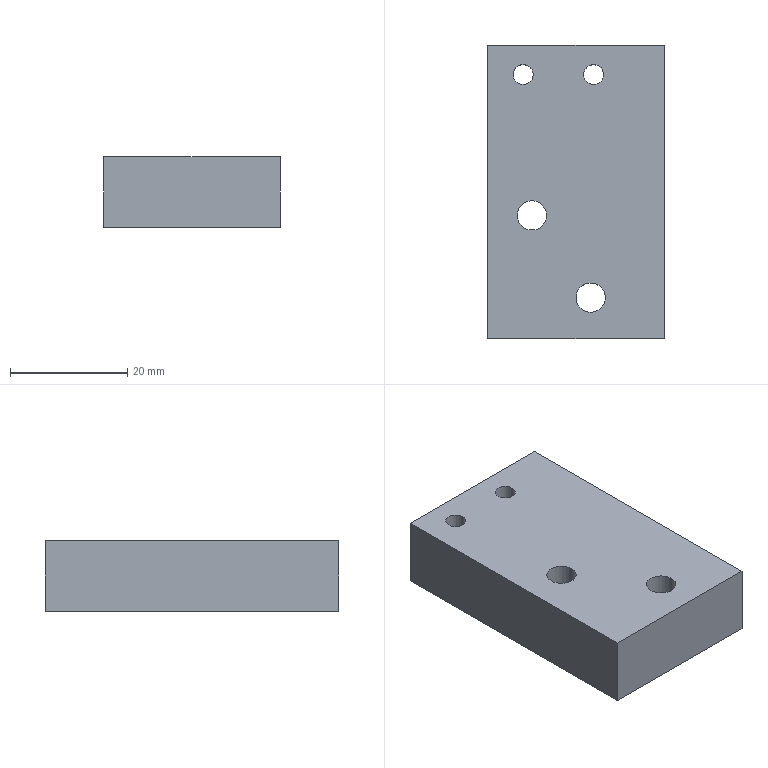Part | SolidWorks | features HoleWzd 2, Extrusion 1, LPattern 1 | 1 solid | 20 faces | box 30 x 50 x 12 mm | volume 17166 mm3 | cylinder 12 | plane 8 | commonest cylinder face diameters 3.4 x4 5 x4 6.5 x4
STEP:
#1=CARTESIAN_POINT('',(6.25,20.,3.));
#2=VERTEX_POINT('',#1);
#3=CARTESIAN_POINT('',(-0.25,20.,3.));
#4=VERTEX_POINT('',#3);
#5=CARTESIAN_POINT('',(3.,20.,3.));
#6=DIRECTION('',(0.,0.,-1.));
#7=DIRECTION('',(-1.,0.,0.));
#8=AXIS2_PLACEMENT_3D('',#5,#6,#7);
#9=CIRCLE('',#8,3.25);
#10=EDGE_CURVE('',#2,#4,#9,.T.);
#11=ORIENTED_EDGE('',*,*,#10,.F.);
#12=CARTESIAN_POINT('',(6.25,20.,0.));
#13=VERTEX_POINT('',#12);
#14=CARTESIAN_POINT('',(6.25,20.,0.));
#15=DIRECTION('',(0.,0.,-1.));
#16=VECTOR('',#15,1000.);
#17=LINE('',#14,#16);
#18=EDGE_CURVE('',#2,#13,#17,.T.);
#19=ORIENTED_EDGE('',*,*,#18,.T.);
#20=CARTESIAN_POINT('',(-0.25,20.,0.));
#21=VERTEX_POINT('',#20);
#22=CARTESIAN_POINT('',(3.,20.,0.));
#23=DIRECTION('',(0.,0.,-1.));
#24=DIRECTION('',(-1.,0.,0.));
#25=AXIS2_PLACEMENT_3D('',#22,#23,#24);
#26=CIRCLE('',#25,3.25);
#27=EDGE_CURVE('',#13,#21,#26,.T.);
#28=ORIENTED_EDGE('',*,*,#27,.T.);
#29=CARTESIAN_POINT('',(-0.25,20.,0.));
#30=DIRECTION('',(0.,0.,-1.));
#31=VECTOR('',#30,1000.);
#32=LINE('',#29,#31);
#33=EDGE_CURVE('',#4,#21,#32,.T.);
#34=ORIENTED_EDGE('',*,*,#33,.F.);
#35=EDGE_LOOP('',(#11,#19,#28,#34));
#36=FACE_OUTER_BOUND('',#35,.T.);
#37=CARTESIAN_POINT('',(3.,20.,0.));
#38=DIRECTION('',(0.,0.,-1.));
#39=DIRECTION('',(-1.,0.,0.));
#40=AXIS2_PLACEMENT_3D('',#37,#38,#39);
#41=CYLINDRICAL_SURFACE('',#40,3.25);
#42=ADVANCED_FACE('',(#36),#41,.F.);
#43=CARTESIAN_POINT('',(4.7,20.,12.));
#44=VERTEX_POINT('',#43);
#45=CARTESIAN_POINT('',(1.3,20.,12.));
#46=VERTEX_POINT('',#45);
#47=CARTESIAN_POINT('',(3.,20.,12.));
#48=DIRECTION('',(0.,0.,-1.));
#49=DIRECTION('',(-1.,0.,0.));
#50=AXIS2_PLACEMENT_3D('',#47,#48,#49);
#51=CIRCLE('',#50,1.7);
#52=EDGE_CURVE('',#44,#46,#51,.T.);
#53=ORIENTED_EDGE('',*,*,#52,.F.);
#54=CARTESIAN_POINT('',(4.7,20.,3.));
#55=VERTEX_POINT('',#54);
#56=CARTESIAN_POINT('',(4.7,20.,0.));
#57=DIRECTION('',(0.,0.,-1.));
#58=VECTOR('',#57,1000.);
#59=LINE('',#56,#58);
#60=EDGE_CURVE('',#44,#55,#59,.T.);
#61=ORIENTED_EDGE('',*,*,#60,.T.);
#62=CARTESIAN_POINT('',(1.3,20.,3.));
#63=VERTEX_POINT('',#62);
#64=CARTESIAN_POINT('',(3.,20.,3.));
#65=DIRECTION('',(0.,0.,-1.));
#66=DIRECTION('',(-1.,0.,0.));
#67=AXIS2_PLACEMENT_3D('',#64,#65,#66);
#68=CIRCLE('',#67,1.7);
#69=EDGE_CURVE('',#55,#63,#68,.T.);
#70=ORIENTED_EDGE('',*,*,#69,.T.);
#71=CARTESIAN_POINT('',(1.3,20.,0.));
#72=DIRECTION('',(0.,0.,-1.));
#73=VECTOR('',#72,1000.);
#74=LINE('',#71,#73);
#75=EDGE_CURVE('',#46,#63,#74,.T.);
#76=ORIENTED_EDGE('',*,*,#75,.F.);
#77=EDGE_LOOP('',(#53,#61,#70,#76));
#78=FACE_OUTER_BOUND('',#77,.T.);
#79=CARTESIAN_POINT('',(3.,20.,0.));
#80=DIRECTION('',(0.,0.,-1.));
#81=DIRECTION('',(-1.,0.,0.));
#82=AXIS2_PLACEMENT_3D('',#79,#80,#81);
#83=CYLINDRICAL_SURFACE('',#82,1.7);
#84=ADVANCED_FACE('',(#78),#83,.F.);
#85=CARTESIAN_POINT('',(-5.75,20.,3.));
#86=VERTEX_POINT('',#85);
#87=CARTESIAN_POINT('',(-12.25,20.,3.));
#88=VERTEX_POINT('',#87);
#89=CARTESIAN_POINT('',(-9.,20.,3.));
#90=DIRECTION('',(0.,0.,-1.));
#91=DIRECTION('',(-1.,0.,0.));
#92=AXIS2_PLACEMENT_3D('',#89,#90,#91);
#93=CIRCLE('',#92,3.25);
#94=EDGE_CURVE('',#86,#88,#93,.T.);
#95=ORIENTED_EDGE('',*,*,#94,.F.);
#96=CARTESIAN_POINT('',(-5.75,20.,0.));
#97=VERTEX_POINT('',#96);
#98=CARTESIAN_POINT('',(-5.75,20.,0.));
#99=DIRECTION('',(0.,0.,-1.));
#100=VECTOR('',#99,1000.);
#101=LINE('',#98,#100);
#102=EDGE_CURVE('',#86,#97,#101,.T.);
#103=ORIENTED_EDGE('',*,*,#102,.T.);
#104=CARTESIAN_POINT('',(-12.25,20.,0.));
#105=VERTEX_POINT('',#104);
#106=CARTESIAN_POINT('',(-9.,20.,0.));
#107=DIRECTION('',(0.,0.,-1.));
#108=DIRECTION('',(-1.,0.,0.));
#109=AXIS2_PLACEMENT_3D('',#106,#107,#108);
#110=CIRCLE('',#109,3.25);
#111=EDGE_CURVE('',#97,#105,#110,.T.);
#112=ORIENTED_EDGE('',*,*,#111,.T.);
#113=CARTESIAN_POINT('',(-12.25,20.,0.));
#114=DIRECTION('',(0.,0.,-1.));
#115=VECTOR('',#114,1000.);
#116=LINE('',#113,#115);
#117=EDGE_CURVE('',#88,#105,#116,.T.);
#118=ORIENTED_EDGE('',*,*,#117,.F.);
#119=EDGE_LOOP('',(#95,#103,#112,#118));
#120=FACE_OUTER_BOUND('',#119,.T.);
#121=CARTESIAN_POINT('',(-9.,20.,0.));
#122=DIRECTION('',(0.,0.,-1.));
#123=DIRECTION('',(-1.,0.,0.));
#124=AXIS2_PLACEMENT_3D('',#121,#122,#123);
#125=CYLINDRICAL_SURFACE('',#124,3.25);
#126=ADVANCED_FACE('',(#120),#125,.F.);
#127=CARTESIAN_POINT('',(-7.3,20.,12.));
#128=VERTEX_POINT('',#127);
#129=CARTESIAN_POINT('',(-10.7,20.,12.));
#130=VERTEX_POINT('',#129);
#131=CARTESIAN_POINT('',(-9.,20.,12.));
#132=DIRECTION('',(0.,0.,-1.));
#133=DIRECTION('',(-1.,0.,0.));
#134=AXIS2_PLACEMENT_3D('',#131,#132,#133);
#135=CIRCLE('',#134,1.7);
#136=EDGE_CURVE('',#128,#130,#135,.T.);
#137=ORIENTED_EDGE('',*,*,#136,.F.);
#138=CARTESIAN_POINT('',(-7.3,20.,3.));
#139=VERTEX_POINT('',#138);
#140=CARTESIAN_POINT('',(-7.3,20.,0.));
#141=DIRECTION('',(0.,0.,-1.));
#142=VECTOR('',#141,1000.);
#143=LINE('',#140,#142);
#144=EDGE_CURVE('',#128,#139,#143,.T.);
#145=ORIENTED_EDGE('',*,*,#144,.T.);
#146=CARTESIAN_POINT('',(-10.7,20.,3.));
#147=VERTEX_POINT('',#146);
#148=CARTESIAN_POINT('',(-9.,20.,3.));
#149=DIRECTION('',(0.,0.,-1.));
#150=DIRECTION('',(-1.,0.,0.));
#151=AXIS2_PLACEMENT_3D('',#148,#149,#150);
#152=CIRCLE('',#151,1.7);
#153=EDGE_CURVE('',#139,#147,#152,.T.);
#154=ORIENTED_EDGE('',*,*,#153,.T.);
#155=CARTESIAN_POINT('',(-10.7,20.,0.));
#156=DIRECTION('',(0.,0.,-1.));
#157=VECTOR('',#156,1000.);
#158=LINE('',#155,#157);
#159=EDGE_CURVE('',#130,#147,#158,.T.);
#160=ORIENTED_EDGE('',*,*,#159,.F.);
#161=EDGE_LOOP('',(#137,#145,#154,#160));
#162=FACE_OUTER_BOUND('',#161,.T.);
#163=CARTESIAN_POINT('',(-9.,20.,0.));
#164=DIRECTION('',(0.,0.,-1.));
#165=DIRECTION('',(-1.,0.,0.));
#166=AXIS2_PLACEMENT_3D('',#163,#164,#165);
#167=CYLINDRICAL_SURFACE('',#166,1.7);
#168=ADVANCED_FACE('',(#162),#167,.F.);
#169=CARTESIAN_POINT('',(-5.,-4.,12.));
#170=VERTEX_POINT('',#169);
#171=CARTESIAN_POINT('',(-10.,-4.,12.));
#172=VERTEX_POINT('',#171);
#173=CARTESIAN_POINT('',(-7.5,-4.,12.));
#174=DIRECTION('',(0.,0.,-1.));
#175=DIRECTION('',(-1.,0.,0.));
#176=AXIS2_PLACEMENT_3D('',#173,#174,#175);
#177=CIRCLE('',#176,2.5);
#178=EDGE_CURVE('',#170,#172,#177,.T.);
#179=ORIENTED_EDGE('',*,*,#178,.F.);
#180=CARTESIAN_POINT('',(-5.,-4.,0.));
#181=VERTEX_POINT('',#180);
#182=CARTESIAN_POINT('',(-5.,-4.,0.));
#183=DIRECTION('',(0.,0.,-1.));
#184=VECTOR('',#183,1000.);
#185=LINE('',#182,#184);
#186=EDGE_CURVE('',#170,#181,#185,.T.);
#187=ORIENTED_EDGE('',*,*,#186,.T.);
#188=CARTESIAN_POINT('',(-10.,-4.,0.));
#189=VERTEX_POINT('',#188);
#190=CARTESIAN_POINT('',(-7.5,-4.,0.));
#191=DIRECTION('',(0.,0.,-1.));
#192=DIRECTION('',(-1.,0.,0.));
#193=AXIS2_PLACEMENT_3D('',#190,#191,#192);
#194=CIRCLE('',#193,2.5);
#195=EDGE_CURVE('',#181,#189,#194,.T.);
#196=ORIENTED_EDGE('',*,*,#195,.T.);
#197=CARTESIAN_POINT('',(-10.,-4.,0.));
#198=DIRECTION('',(0.,0.,-1.));
#199=VECTOR('',#198,1000.);
#200=LINE('',#197,#199);
#201=EDGE_CURVE('',#172,#189,#200,.T.);
#202=ORIENTED_EDGE('',*,*,#201,.F.);
#203=EDGE_LOOP('',(#179,#187,#196,#202));
#204=FACE_OUTER_BOUND('',#203,.T.);
#205=CARTESIAN_POINT('',(-7.5,-4.,0.));
#206=DIRECTION('',(0.,0.,-1.));
#207=DIRECTION('',(-1.,0.,0.));
#208=AXIS2_PLACEMENT_3D('',#205,#206,#207);
#209=CYLINDRICAL_SURFACE('',#208,2.5);
#210=ADVANCED_FACE('',(#204),#209,.F.);
#211=CARTESIAN_POINT('',(5.,-18.,12.));
#212=VERTEX_POINT('',#211);
#213=CARTESIAN_POINT('',(0.,-18.,12.));
#214=VERTEX_POINT('',#213);
#215=CARTESIAN_POINT('',(2.5,-18.,12.));
#216=DIRECTION('',(0.,0.,-1.));
#217=DIRECTION('',(-1.,0.,0.));
#218=AXIS2_PLACEMENT_3D('',#215,#216,#217);
#219=CIRCLE('',#218,2.5);
#220=EDGE_CURVE('',#212,#214,#219,.T.);
#221=ORIENTED_EDGE('',*,*,#220,.F.);
#222=CARTESIAN_POINT('',(5.,-18.,0.));
#223=VERTEX_POINT('',#222);
#224=CARTESIAN_POINT('',(5.,-18.,0.));
#225=DIRECTION('',(0.,0.,-1.));
#226=VECTOR('',#225,1000.);
#227=LINE('',#224,#226);
#228=EDGE_CURVE('',#212,#223,#227,.T.);
#229=ORIENTED_EDGE('',*,*,#228,.T.);
#230=CARTESIAN_POINT('',(0.,-18.,0.));
#231=VERTEX_POINT('',#230);
#232=CARTESIAN_POINT('',(2.5,-18.,0.));
#233=DIRECTION('',(0.,0.,-1.));
#234=DIRECTION('',(-1.,0.,0.));
#235=AXIS2_PLACEMENT_3D('',#232,#233,#234);
#236=CIRCLE('',#235,2.5);
#237=EDGE_CURVE('',#223,#231,#236,.T.);
#238=ORIENTED_EDGE('',*,*,#237,.T.);
#239=CARTESIAN_POINT('',(0.,-18.,0.));
#240=DIRECTION('',(0.,0.,-1.));
#241=VECTOR('',#240,1000.);
#242=LINE('',#239,#241);
#243=EDGE_CURVE('',#214,#231,#242,.T.);
#244=ORIENTED_EDGE('',*,*,#243,.F.);
#245=EDGE_LOOP('',(#221,#229,#238,#244));
#246=FACE_OUTER_BOUND('',#245,.T.);
#247=CARTESIAN_POINT('',(2.5,-18.,0.));
#248=DIRECTION('',(0.,0.,-1.));
#249=DIRECTION('',(-1.,0.,0.));
#250=AXIS2_PLACEMENT_3D('',#247,#248,#249);
#251=CYLINDRICAL_SURFACE('',#250,2.5);
#252=ADVANCED_FACE('',(#246),#251,.F.);
#253=CARTESIAN_POINT('',(15.,-25.,0.));
#254=VERTEX_POINT('',#253);
#255=CARTESIAN_POINT('',(15.,25.,0.));
#256=VERTEX_POINT('',#255);
#257=CARTESIAN_POINT('',(15.,-25.,0.));
#258=DIRECTION('',(0.,1.,0.));
#259=VECTOR('',#258,1000.);
#260=LINE('',#257,#259);
#261=EDGE_CURVE('',#254,#256,#260,.T.);
#262=ORIENTED_EDGE('',*,*,#261,.T.);
#263=CARTESIAN_POINT('',(15.,25.,12.));
#264=VERTEX_POINT('',#263);
#265=CARTESIAN_POINT('',(15.,25.,12.));
#266=DIRECTION('',(0.,0.,-1.));
#267=VECTOR('',#266,1000.);
#268=LINE('',#265,#267);
#269=EDGE_CURVE('',#264,#256,#268,.T.);
#270=ORIENTED_EDGE('',*,*,#269,.F.);
#271=CARTESIAN_POINT('',(15.,-25.,12.));
#272=VERTEX_POINT('',#271);
#273=CARTESIAN_POINT('',(15.,-25.,12.));
#274=DIRECTION('',(0.,1.,0.));
#275=VECTOR('',#274,1000.);
#276=LINE('',#273,#275);
#277=EDGE_CURVE('',#272,#264,#276,.T.);
#278=ORIENTED_EDGE('',*,*,#277,.F.);
#279=CARTESIAN_POINT('',(15.,-25.,12.));
#280=DIRECTION('',(0.,0.,-1.));
#281=VECTOR('',#280,1000.);
#282=LINE('',#279,#281);
#283=EDGE_CURVE('',#272,#254,#282,.T.);
#284=ORIENTED_EDGE('',*,*,#283,.T.);
#285=EDGE_LOOP('',(#262,#270,#278,#284));
#286=FACE_OUTER_BOUND('',#285,.T.);
#287=CARTESIAN_POINT('',(15.,-25.,12.));
#288=DIRECTION('',(-1.,0.,0.));
#289=DIRECTION('',(0.,0.,1.));
#290=AXIS2_PLACEMENT_3D('',#287,#288,#289);
#291=PLANE('',#290);
#292=ADVANCED_FACE('',(#286),#291,.F.);
#293=CARTESIAN_POINT('',(-15.,25.,0.));
#294=VERTEX_POINT('',#293);
#295=CARTESIAN_POINT('',(-15.,25.,0.));
#296=DIRECTION('',(-1.,0.,0.));
#297=VECTOR('',#296,1000.);
#298=LINE('',#295,#297);
#299=EDGE_CURVE('',#256,#294,#298,.T.);
#300=ORIENTED_EDGE('',*,*,#299,.T.);
#301=CARTESIAN_POINT('',(-15.,25.,12.));
#302=VERTEX_POINT('',#301);
#303=CARTESIAN_POINT('',(-15.,25.,12.));
#304=DIRECTION('',(0.,0.,-1.));
#305=VECTOR('',#304,1000.);
#306=LINE('',#303,#305);
#307=EDGE_CURVE('',#302,#294,#306,.T.);
#308=ORIENTED_EDGE('',*,*,#307,.F.);
#309=CARTESIAN_POINT('',(-15.,25.,12.));
#310=DIRECTION('',(-1.,0.,0.));
#311=VECTOR('',#310,1000.);
#312=LINE('',#309,#311);
#313=EDGE_CURVE('',#264,#302,#312,.T.);
#314=ORIENTED_EDGE('',*,*,#313,.F.);
#315=ORIENTED_EDGE('',*,*,#269,.T.);
#316=EDGE_LOOP('',(#300,#308,#314,#315));
#317=FACE_OUTER_BOUND('',#316,.T.);
#318=CARTESIAN_POINT('',(-15.,25.,12.));
#319=DIRECTION('',(0.,-1.,0.));
#320=DIRECTION('',(0.,0.,-1.));
#321=AXIS2_PLACEMENT_3D('',#318,#319,#320);
#322=PLANE('',#321);
#323=ADVANCED_FACE('',(#317),#322,.F.);
#324=CARTESIAN_POINT('',(-15.,-25.,0.));
#325=VERTEX_POINT('',#324);
#326=CARTESIAN_POINT('',(-15.,-25.,0.));
#327=DIRECTION('',(0.,-1.,0.));
#328=VECTOR('',#327,1000.);
#329=LINE('',#326,#328);
#330=EDGE_CURVE('',#294,#325,#329,.T.);
#331=ORIENTED_EDGE('',*,*,#330,.T.);
#332=CARTESIAN_POINT('',(-15.,-25.,12.));
#333=VERTEX_POINT('',#332);
#334=CARTESIAN_POINT('',(-15.,-25.,12.));
#335=DIRECTION('',(0.,0.,-1.));
#336=VECTOR('',#335,1000.);
#337=LINE('',#334,#336);
#338=EDGE_CURVE('',#333,#325,#337,.T.);
#339=ORIENTED_EDGE('',*,*,#338,.F.);
#340=CARTESIAN_POINT('',(-15.,-25.,12.));
#341=DIRECTION('',(0.,-1.,0.));
#342=VECTOR('',#341,1000.);
#343=LINE('',#340,#342);
#344=EDGE_CURVE('',#302,#333,#343,.T.);
#345=ORIENTED_EDGE('',*,*,#344,.F.);
#346=ORIENTED_EDGE('',*,*,#307,.T.);
#347=EDGE_LOOP('',(#331,#339,#345,#346));
#348=FACE_OUTER_BOUND('',#347,.T.);
#349=CARTESIAN_POINT('',(-15.,-25.,12.));
#350=DIRECTION('',(1.,0.,0.));
#351=DIRECTION('',(0.,0.,-1.));
#352=AXIS2_PLACEMENT_3D('',#349,#350,#351);
#353=PLANE('',#352);
#354=ADVANCED_FACE('',(#348),#353,.F.);
#355=CARTESIAN_POINT('',(-15.,-25.,0.));
#356=DIRECTION('',(1.,0.,0.));
#357=VECTOR('',#356,1000.);
#358=LINE('',#355,#357);
#359=EDGE_CURVE('',#325,#254,#358,.T.);
#360=ORIENTED_EDGE('',*,*,#359,.T.);
#361=ORIENTED_EDGE('',*,*,#283,.F.);
#362=CARTESIAN_POINT('',(-15.,-25.,12.));
#363=DIRECTION('',(1.,0.,0.));
#364=VECTOR('',#363,1000.);
#365=LINE('',#362,#364);
#366=EDGE_CURVE('',#333,#272,#365,.T.);
#367=ORIENTED_EDGE('',*,*,#366,.F.);
#368=ORIENTED_EDGE('',*,*,#338,.T.);
#369=EDGE_LOOP('',(#360,#361,#367,#368));
#370=FACE_OUTER_BOUND('',#369,.T.);
#371=CARTESIAN_POINT('',(-15.,-25.,12.));
#372=DIRECTION('',(0.,1.,0.));
#373=DIRECTION('',(0.,0.,1.));
#374=AXIS2_PLACEMENT_3D('',#371,#372,#373);
#375=PLANE('',#374);
#376=ADVANCED_FACE('',(#370),#375,.F.);
#377=CARTESIAN_POINT('',(3.,20.,12.));
#378=DIRECTION('',(0.,0.,-1.));
#379=DIRECTION('',(-1.,0.,0.));
#380=AXIS2_PLACEMENT_3D('',#377,#378,#379);
#381=CIRCLE('',#380,1.7);
#382=EDGE_CURVE('',#46,#44,#381,.T.);
#383=ORIENTED_EDGE('',*,*,#382,.T.);
#384=ORIENTED_EDGE('',*,*,#52,.T.);
#385=EDGE_LOOP('',(#383,#384));
#386=FACE_BOUND('',#385,.T.);
#387=CARTESIAN_POINT('',(-9.,20.,12.));
#388=DIRECTION('',(0.,0.,-1.));
#389=DIRECTION('',(-1.,0.,0.));
#390=AXIS2_PLACEMENT_3D('',#387,#388,#389);
#391=CIRCLE('',#390,1.7);
#392=EDGE_CURVE('',#130,#128,#391,.T.);
#393=ORIENTED_EDGE('',*,*,#392,.T.);
#394=ORIENTED_EDGE('',*,*,#136,.T.);
#395=EDGE_LOOP('',(#393,#394));
#396=FACE_BOUND('',#395,.T.);
#397=CARTESIAN_POINT('',(-7.5,-4.,12.));
#398=DIRECTION('',(0.,0.,-1.));
#399=DIRECTION('',(-1.,0.,0.));
#400=AXIS2_PLACEMENT_3D('',#397,#398,#399);
#401=CIRCLE('',#400,2.5);
#402=EDGE_CURVE('',#172,#170,#401,.T.);
#403=ORIENTED_EDGE('',*,*,#402,.T.);
#404=ORIENTED_EDGE('',*,*,#178,.T.);
#405=EDGE_LOOP('',(#403,#404));
#406=FACE_BOUND('',#405,.T.);
#407=CARTESIAN_POINT('',(2.5,-18.,12.));
#408=DIRECTION('',(0.,0.,-1.));
#409=DIRECTION('',(-1.,0.,0.));
#410=AXIS2_PLACEMENT_3D('',#407,#408,#409);
#411=CIRCLE('',#410,2.5);
#412=EDGE_CURVE('',#214,#212,#411,.T.);
#413=ORIENTED_EDGE('',*,*,#412,.T.);
#414=ORIENTED_EDGE('',*,*,#220,.T.);
#415=EDGE_LOOP('',(#413,#414));
#416=FACE_BOUND('',#415,.T.);
#417=ORIENTED_EDGE('',*,*,#277,.T.);
#418=ORIENTED_EDGE('',*,*,#313,.T.);
#419=ORIENTED_EDGE('',*,*,#344,.T.);
#420=ORIENTED_EDGE('',*,*,#366,.T.);
#421=EDGE_LOOP('',(#417,#418,#419,#420));
#422=FACE_OUTER_BOUND('',#421,.T.);
#423=CARTESIAN_POINT('',(15.,25.,12.));
#424=DIRECTION('',(0.,0.,-1.));
#425=DIRECTION('',(-1.,0.,0.));
#426=AXIS2_PLACEMENT_3D('',#423,#424,#425);
#427=PLANE('',#426);
#428=ADVANCED_FACE('',(#386,#396,#406,#416,#422),#427,.F.);
#429=CARTESIAN_POINT('',(3.,20.,0.));
#430=DIRECTION('',(0.,0.,-1.));
#431=DIRECTION('',(-1.,0.,0.));
#432=AXIS2_PLACEMENT_3D('',#429,#430,#431);
#433=CIRCLE('',#432,3.25);
#434=EDGE_CURVE('',#21,#13,#433,.T.);
#435=ORIENTED_EDGE('',*,*,#434,.F.);
#436=ORIENTED_EDGE('',*,*,#27,.F.);
#437=EDGE_LOOP('',(#435,#436));
#438=FACE_BOUND('',#437,.T.);
#439=CARTESIAN_POINT('',(-9.,20.,0.));
#440=DIRECTION('',(0.,0.,-1.));
#441=DIRECTION('',(-1.,0.,0.));
#442=AXIS2_PLACEMENT_3D('',#439,#440,#441);
#443=CIRCLE('',#442,3.25);
#444=EDGE_CURVE('',#105,#97,#443,.T.);
#445=ORIENTED_EDGE('',*,*,#444,.F.);
#446=ORIENTED_EDGE('',*,*,#111,.F.);
#447=EDGE_LOOP('',(#445,#446));
#448=FACE_BOUND('',#447,.T.);
#449=CARTESIAN_POINT('',(-7.5,-4.,0.));
#450=DIRECTION('',(0.,0.,-1.));
#451=DIRECTION('',(-1.,0.,0.));
#452=AXIS2_PLACEMENT_3D('',#449,#450,#451);
#453=CIRCLE('',#452,2.5);
#454=EDGE_CURVE('',#189,#181,#453,.T.);
#455=ORIENTED_EDGE('',*,*,#454,.F.);
#456=ORIENTED_EDGE('',*,*,#195,.F.);
#457=EDGE_LOOP('',(#455,#456));
#458=FACE_BOUND('',#457,.T.);
#459=CARTESIAN_POINT('',(2.5,-18.,0.));
#460=DIRECTION('',(0.,0.,-1.));
#461=DIRECTION('',(-1.,0.,0.));
#462=AXIS2_PLACEMENT_3D('',#459,#460,#461);
#463=CIRCLE('',#462,2.5);
#464=EDGE_CURVE('',#231,#223,#463,.T.);
#465=ORIENTED_EDGE('',*,*,#464,.F.);
#466=ORIENTED_EDGE('',*,*,#237,.F.);
#467=EDGE_LOOP('',(#465,#466));
#468=FACE_BOUND('',#467,.T.);
#469=ORIENTED_EDGE('',*,*,#261,.F.);
#470=ORIENTED_EDGE('',*,*,#359,.F.);
#471=ORIENTED_EDGE('',*,*,#330,.F.);
#472=ORIENTED_EDGE('',*,*,#299,.F.);
#473=EDGE_LOOP('',(#469,#470,#471,#472));
#474=FACE_OUTER_BOUND('',#473,.T.);
#475=CARTESIAN_POINT('',(15.,25.,0.));
#476=DIRECTION('',(0.,0.,-1.));
#477=DIRECTION('',(-1.,0.,0.));
#478=AXIS2_PLACEMENT_3D('',#475,#476,#477);
#479=PLANE('',#478);
#480=ADVANCED_FACE('',(#438,#448,#458,#468,#474),#479,.T.);
#481=ORIENTED_EDGE('',*,*,#228,.F.);
#482=ORIENTED_EDGE('',*,*,#412,.F.);
#483=ORIENTED_EDGE('',*,*,#243,.T.);
#484=ORIENTED_EDGE('',*,*,#464,.T.);
#485=EDGE_LOOP('',(#481,#482,#483,#484));
#486=FACE_OUTER_BOUND('',#485,.T.);
#487=CARTESIAN_POINT('',(2.5,-18.,0.));
#488=DIRECTION('',(0.,0.,-1.));
#489=DIRECTION('',(-1.,0.,0.));
#490=AXIS2_PLACEMENT_3D('',#487,#488,#489);
#491=CYLINDRICAL_SURFACE('',#490,2.5);
#492=ADVANCED_FACE('',(#486),#491,.F.);
#493=ORIENTED_EDGE('',*,*,#186,.F.);
#494=ORIENTED_EDGE('',*,*,#402,.F.);
#495=ORIENTED_EDGE('',*,*,#201,.T.);
#496=ORIENTED_EDGE('',*,*,#454,.T.);
#497=EDGE_LOOP('',(#493,#494,#495,#496));
#498=FACE_OUTER_BOUND('',#497,.T.);
#499=CARTESIAN_POINT('',(-7.5,-4.,0.));
#500=DIRECTION('',(0.,0.,-1.));
#501=DIRECTION('',(-1.,0.,0.));
#502=AXIS2_PLACEMENT_3D('',#499,#500,#501);
#503=CYLINDRICAL_SURFACE('',#502,2.5);
#504=ADVANCED_FACE('',(#498),#503,.F.);
#505=ORIENTED_EDGE('',*,*,#144,.F.);
#506=ORIENTED_EDGE('',*,*,#392,.F.);
#507=ORIENTED_EDGE('',*,*,#159,.T.);
#508=CARTESIAN_POINT('',(-9.,20.,3.));
#509=DIRECTION('',(0.,0.,-1.));
#510=DIRECTION('',(-1.,0.,0.));
#511=AXIS2_PLACEMENT_3D('',#508,#509,#510);
#512=CIRCLE('',#511,1.7);
#513=EDGE_CURVE('',#147,#139,#512,.T.);
#514=ORIENTED_EDGE('',*,*,#513,.T.);
#515=EDGE_LOOP('',(#505,#506,#507,#514));
#516=FACE_OUTER_BOUND('',#515,.T.);
#517=CARTESIAN_POINT('',(-9.,20.,0.));
#518=DIRECTION('',(0.,0.,-1.));
#519=DIRECTION('',(-1.,0.,0.));
#520=AXIS2_PLACEMENT_3D('',#517,#518,#519);
#521=CYLINDRICAL_SURFACE('',#520,1.7);
#522=ADVANCED_FACE('',(#516),#521,.F.);
#523=ORIENTED_EDGE('',*,*,#513,.F.);
#524=ORIENTED_EDGE('',*,*,#153,.F.);
#525=EDGE_LOOP('',(#523,#524));
#526=FACE_BOUND('',#525,.T.);
#527=CARTESIAN_POINT('',(-9.,20.,3.));
#528=DIRECTION('',(0.,0.,-1.));
#529=DIRECTION('',(-1.,0.,0.));
#530=AXIS2_PLACEMENT_3D('',#527,#528,#529);
#531=CIRCLE('',#530,3.25);
#532=EDGE_CURVE('',#88,#86,#531,.T.);
#533=ORIENTED_EDGE('',*,*,#532,.T.);
#534=ORIENTED_EDGE('',*,*,#94,.T.);
#535=EDGE_LOOP('',(#533,#534));
#536=FACE_OUTER_BOUND('',#535,.T.);
#537=CARTESIAN_POINT('',(-7.3,20.,3.));
#538=DIRECTION('',(0.,0.,1.));
#539=DIRECTION('',(1.,0.,0.));
#540=AXIS2_PLACEMENT_3D('',#537,#538,#539);
#541=PLANE('',#540);
#542=ADVANCED_FACE('',(#526,#536),#541,.F.);
#543=ORIENTED_EDGE('',*,*,#102,.F.);
#544=ORIENTED_EDGE('',*,*,#532,.F.);
#545=ORIENTED_EDGE('',*,*,#117,.T.);
#546=ORIENTED_EDGE('',*,*,#444,.T.);
#547=EDGE_LOOP('',(#543,#544,#545,#546));
#548=FACE_OUTER_BOUND('',#547,.T.);
#549=CARTESIAN_POINT('',(-9.,20.,0.));
#550=DIRECTION('',(0.,0.,-1.));
#551=DIRECTION('',(-1.,0.,0.));
#552=AXIS2_PLACEMENT_3D('',#549,#550,#551);
#553=CYLINDRICAL_SURFACE('',#552,3.25);
#554=ADVANCED_FACE('',(#548),#553,.F.);
#555=ORIENTED_EDGE('',*,*,#18,.F.);
#556=CARTESIAN_POINT('',(3.,20.,3.));
#557=DIRECTION('',(0.,0.,-1.));
#558=DIRECTION('',(-1.,0.,0.));
#559=AXIS2_PLACEMENT_3D('',#556,#557,#558);
#560=CIRCLE('',#559,3.25);
#561=EDGE_CURVE('',#4,#2,#560,.T.);
#562=ORIENTED_EDGE('',*,*,#561,.F.);
#563=ORIENTED_EDGE('',*,*,#33,.T.);
#564=ORIENTED_EDGE('',*,*,#434,.T.);
#565=EDGE_LOOP('',(#555,#562,#563,#564));
#566=FACE_OUTER_BOUND('',#565,.T.);
#567=CARTESIAN_POINT('',(3.,20.,0.));
#568=DIRECTION('',(0.,0.,-1.));
#569=DIRECTION('',(-1.,0.,0.));
#570=AXIS2_PLACEMENT_3D('',#567,#568,#569);
#571=CYLINDRICAL_SURFACE('',#570,3.25);
#572=ADVANCED_FACE('',(#566),#571,.F.);
#573=CARTESIAN_POINT('',(3.,20.,3.));
#574=DIRECTION('',(0.,0.,-1.));
#575=DIRECTION('',(-1.,0.,0.));
#576=AXIS2_PLACEMENT_3D('',#573,#574,#575);
#577=CIRCLE('',#576,1.7);
#578=EDGE_CURVE('',#63,#55,#577,.T.);
#579=ORIENTED_EDGE('',*,*,#578,.F.);
#580=ORIENTED_EDGE('',*,*,#69,.F.);
#581=EDGE_LOOP('',(#579,#580));
#582=FACE_BOUND('',#581,.T.);
#583=ORIENTED_EDGE('',*,*,#561,.T.);
#584=ORIENTED_EDGE('',*,*,#10,.T.);
#585=EDGE_LOOP('',(#583,#584));
#586=FACE_OUTER_BOUND('',#585,.T.);
#587=CARTESIAN_POINT('',(4.7,20.,3.));
#588=DIRECTION('',(0.,0.,1.));
#589=DIRECTION('',(1.,0.,0.));
#590=AXIS2_PLACEMENT_3D('',#587,#588,#589);
#591=PLANE('',#590);
#592=ADVANCED_FACE('',(#582,#586),#591,.F.);
#593=ORIENTED_EDGE('',*,*,#60,.F.);
#594=ORIENTED_EDGE('',*,*,#382,.F.);
#595=ORIENTED_EDGE('',*,*,#75,.T.);
#596=ORIENTED_EDGE('',*,*,#578,.T.);
#597=EDGE_LOOP('',(#593,#594,#595,#596));
#598=FACE_OUTER_BOUND('',#597,.T.);
#599=CARTESIAN_POINT('',(3.,20.,0.));
#600=DIRECTION('',(0.,0.,-1.));
#601=DIRECTION('',(-1.,0.,0.));
#602=AXIS2_PLACEMENT_3D('',#599,#600,#601);
#603=CYLINDRICAL_SURFACE('',#602,1.7);
#604=ADVANCED_FACE('',(#598),#603,.F.);
#605=CLOSED_SHELL('',(#42,#84,#126,#168,#210,#252,#292,#323,#354,#376,#428,#480,#492,#504,#522,#542,#554,#572,#592,#604));
#606=MANIFOLD_SOLID_BREP('',#605);
#607=CARTESIAN_POINT('',(0.,0.,0.));
#608=DIRECTION('',(0.,0.,1.));
#609=DIRECTION('',(1.,0.,0.));
#610=AXIS2_PLACEMENT_3D('',#607,#608,#609);
#611=(LENGTH_UNIT()NAMED_UNIT(*)SI_UNIT(.MILLI.,.METRE.));
#612=UNCERTAINTY_MEASURE_WITH_UNIT(LENGTH_MEASURE(0.00001),#611,'','');
#613=(NAMED_UNIT(*)PLANE_ANGLE_UNIT()SI_UNIT($,.RADIAN.));
#614=(NAMED_UNIT(*)SI_UNIT($,.STERADIAN.)SOLID_ANGLE_UNIT());
#615=(GEOMETRIC_REPRESENTATION_CONTEXT(3)GLOBAL_UNCERTAINTY_ASSIGNED_CONTEXT((#612))GLOBAL_UNIT_ASSIGNED_CONTEXT((#611,#613,#614))REPRESENTATION_CONTEXT('',''));
#616=ADVANCED_BREP_SHAPE_REPRESENTATION('',(#606,#610),#615);